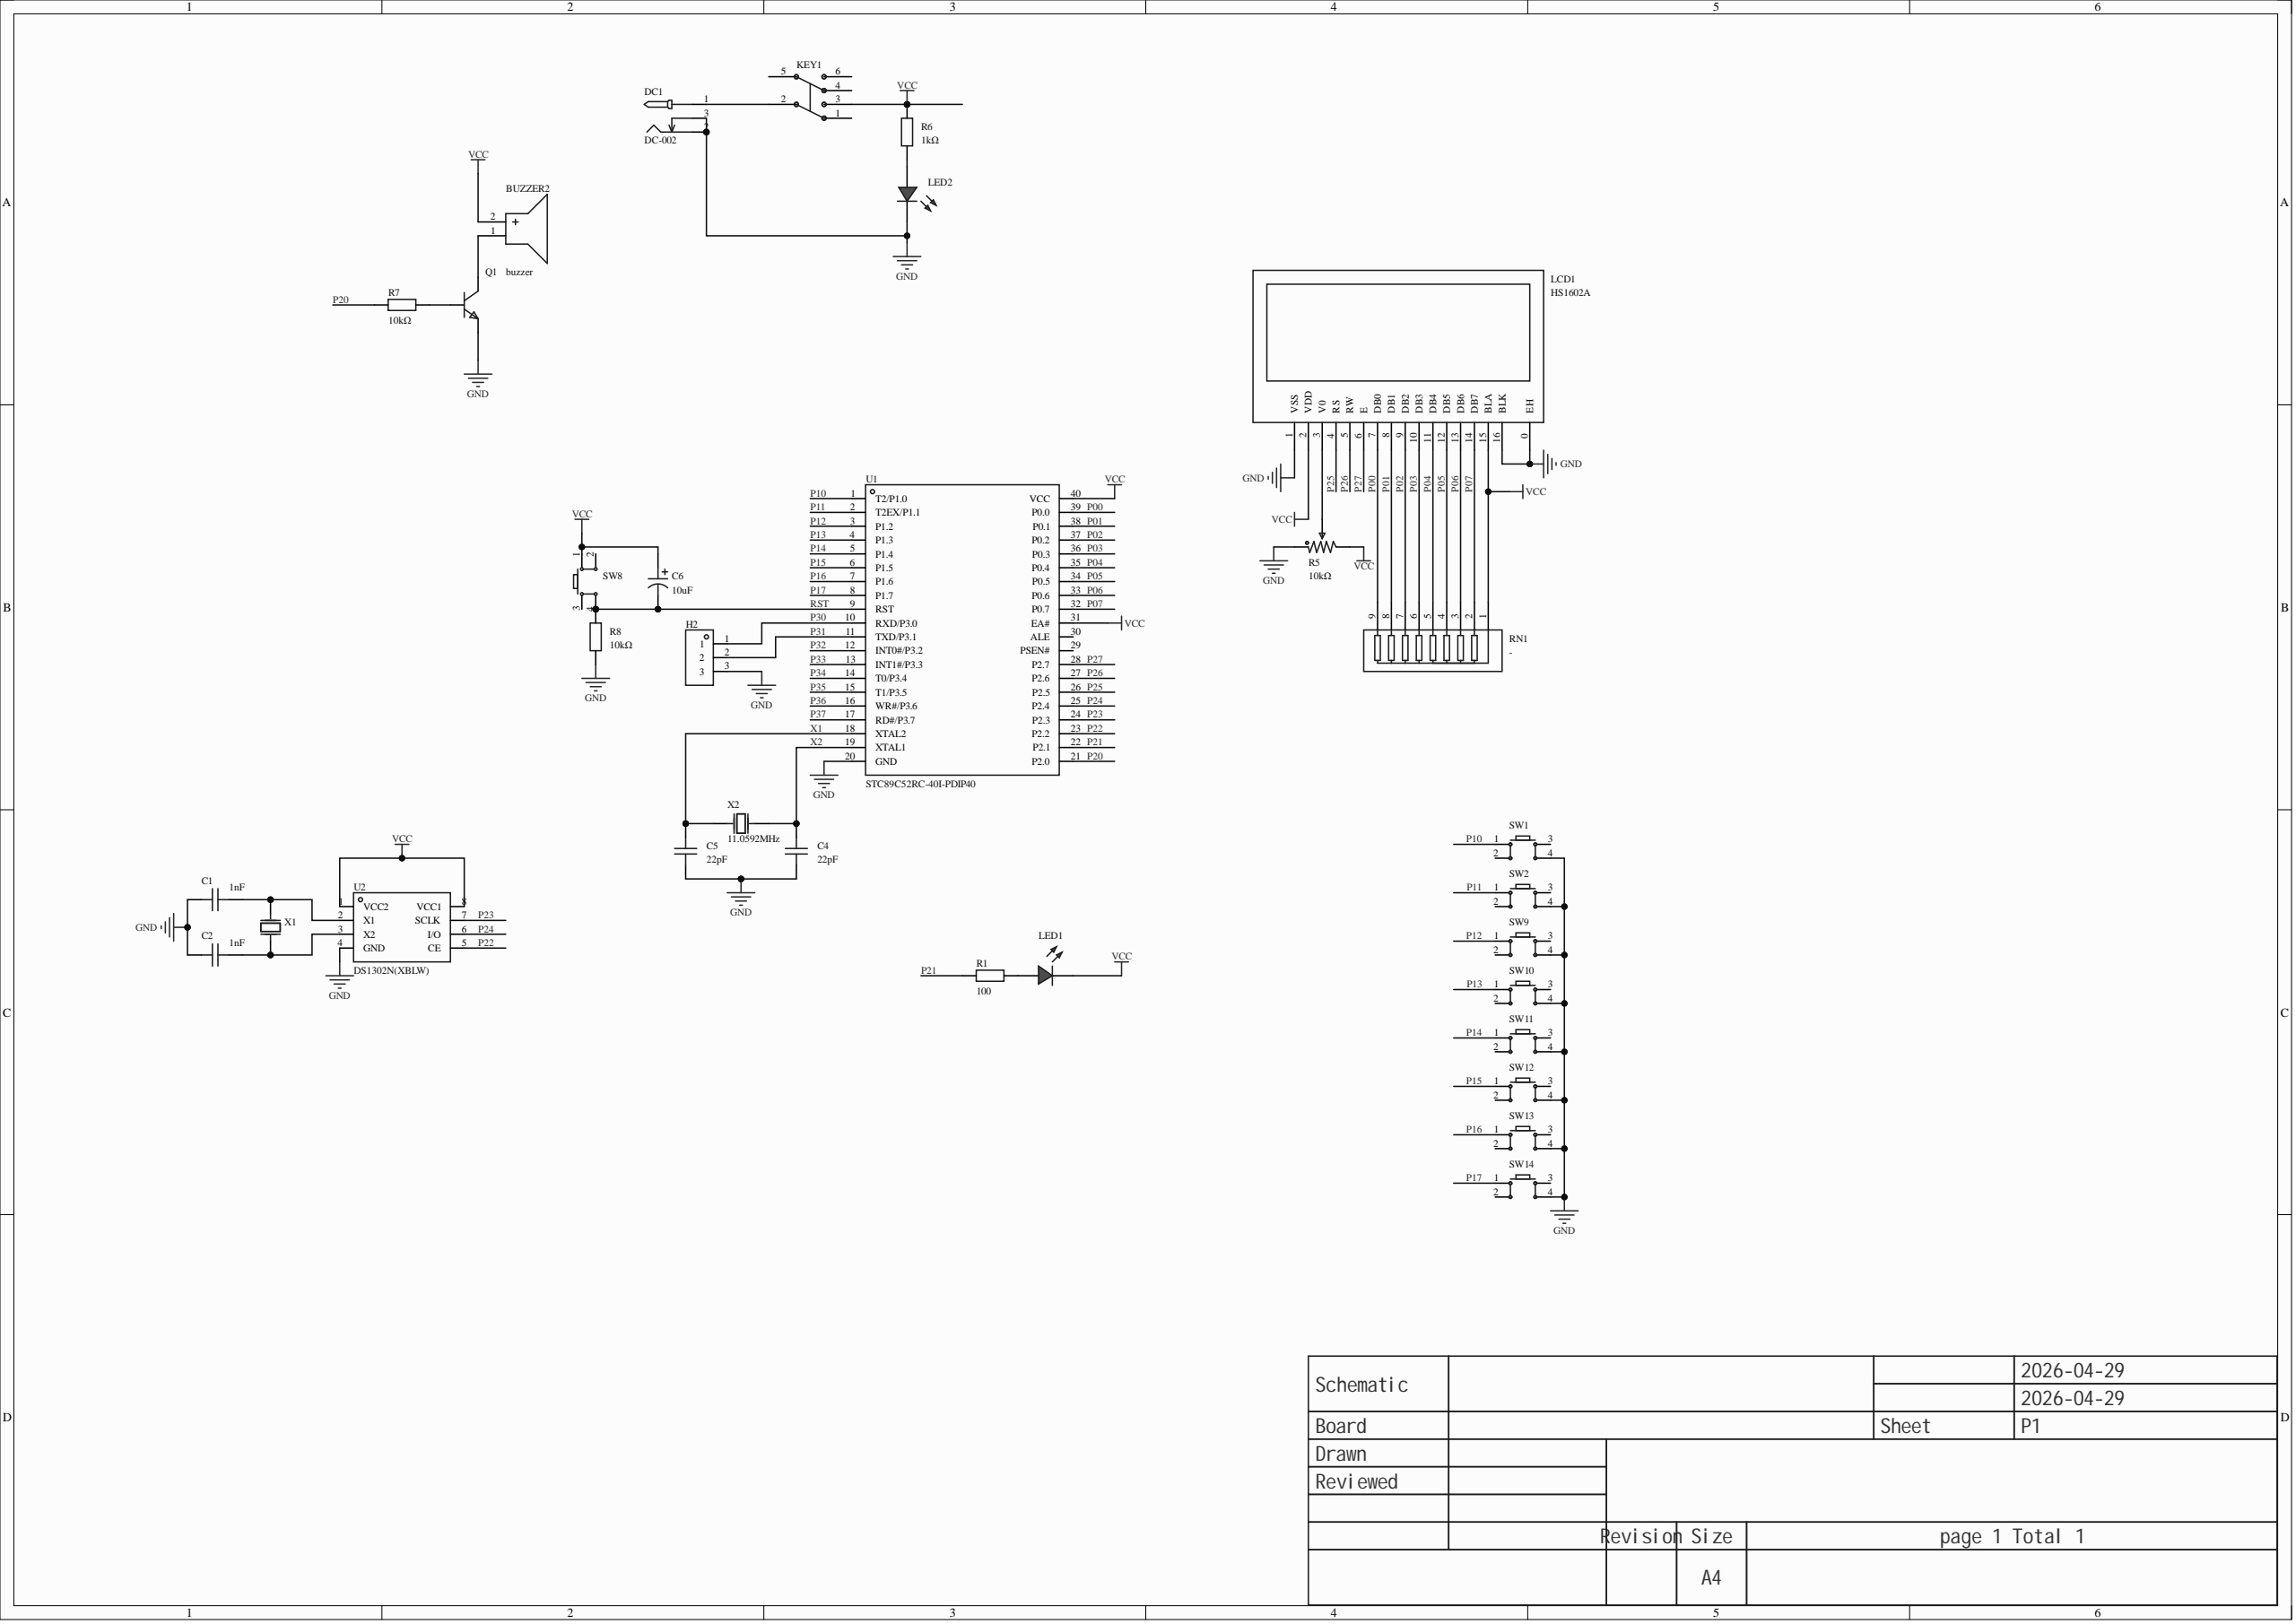Circuit board | Altium Designer | 32 parts | 39 nets
Bill of materials:
Comment,Description,Designator,Footprint,LibRef,Quantity
"buzzer","","BUZZER2","BUZ-TH_BD12.0-P6.00-D0.9-RD","buzzer","1"
"1nF","Capacitance: 30pF; tolerance: ±10%; rated voltage: 25V; temperature coefficient: C0G;","C1, C2","CAP-TH_L3.8-W2.5-P2.54-D0.50","C315C300K3G5TA7301","2"
"22pF","Capacitance: 30pF; tolerance: ±10%; rated voltage: 25V; temperature coefficient: C0G;","C4, C5","CAP-TH_L3.8-W2.5-P2.54-D0.50","C315C300K3G5TA7301","2"
"10uF","Capacitance: 10uF; tolerance: ±20%; rated voltage: 50V; ripple current: 120mA@100KHz; equivalent series resistance (ESR): 1.6Ω;","C6","CAP-TH_BD5.0-P2.00-D0.8-FD-10UF50VC110GL","10UF50VC110GL","1"
"DC-002","","DC1","DC-IN-TH_DC-3510","DC-002","1"
"","","H2","HDR-TH_3P-P2.54-V-M","HDR-M_2.54_1x3P","1"
"Non-latching switch 8.5×8.5 silent","6 pins, 8.5×8.5","KEY1","SW-TH_6P-L8.5-W8.5-P2.54","无自锁开关 8.5×8.5 无声","1"
"HS1602A","Controller chip: SPLC780; size (inch): 2;","LCD1","LCD1602","HS1602A","1"
"","","LED1, LED2","LED_TH-3mm","LED_TH-R_3mm","2"
"","","Q1","S8050_TO_92","S8050_TO_NPN","1"
"100","","R1","Res_1/8W","Res_AXIAL-1/8W","1"
"10kΩ","Resistance: 10kΩ; tolerance: ±25%; power: 100mW;","R5","RES-ADJ-SMD_RM065-V1","RM065-103(10K)","1"
"1kΩ","","R6","Res_1/8W","Res_AXIAL-1/8W","1"
"10kΩ","","R7, R8","Res_1/8W","Res_AXIAL-1/8W","2"
"-","Number of resistors: -; resistance: -; power per element: -;","RN1","RES-ARRAY-TH_9P-P2.54-D1.0","排阻 10 K 5%","1"
"","","SW1, SW2, SW8, SW9, SW10, SW11, SW12, SW13, SW14","SW-TH_4P-L6.0-W6.0-P4.50-LS6.5","Key_TH_6x6x6","9"
"STC89C52RC-40I-PDIP40","CPU core: 51 family; max CPU frequency: -;","U1","DIP-40_L52.0-W13.7-P2.54-LS15.2-BL","STC89C52RC-40I-PDIP40","1"
"DS1302N(XBLW)","Interface type: Three-wire serial interface; crystal: external; alarm output: -;","U2","PDIP-8_L9.3-W6.4-P2.54-LS7.6-BL","DS1302N(XBLW)","1"
"11.059MHz","Crystal type: through-hole crystal; frequency: 11.059MHz; frequency tolerance at room temperature: ±20ppm; load capacitance: 30pF;","X1, X2","OSC-TH_L11.1-W4.7-P4.88","9AC11059302060C3","2"
Netlist (Protel format):
[
BUZZER2
BUZ-TH_BD12.0-P6.00-D0.9-RD
buzzer



]
[
C1
CAP-TH_L3.8-W2.5-P2.54-D0.50
1nF



]
[
C2
CAP-TH_L3.8-W2.5-P2.54-D0.50
1nF



]
[
C4
CAP-TH_L3.8-W2.5-P2.54-D0.50
22pF



]
[
C5
CAP-TH_L3.8-W2.5-P2.54-D0.50
22pF



]
[
C6
CAP-TH_BD5.0-P2.00-D0.8-FD-10UF50VC110GL
10uF



]
[
DC1
DC-IN-TH_DC-3510
DC-002



]
[
H2
HDR-TH_3P-P2.54-V-M




]
[
KEY1
SW-TH_6P-L8.5-W8.5-P2.54
Non-latching switch 8.5×8.5 silent



]
[
LCD1
LCD1602
HS1602A



]
[
LED1
LED_TH-3mm




]
[
LED2
LED_TH-3mm




]
[
Q1
S8050_TO_92




]
[
R1
Res_1/8W
100



]
[
R5
RES-ADJ-SMD_RM065-V1
10kΩ



]
[
R6
Res_1/8W
1kΩ



]
[
R7
Res_1/8W
10kΩ



]
[
R8
Res_1/8W
10kΩ



]
[
RN1
RES-ARRAY-TH_9P-P2.54-D1.0
-



]
[
SW1
SW-TH_4P-L6.0-W6.0-P4.50-LS6.5




]
[
SW2
SW-TH_4P-L6.0-W6.0-P4.50-LS6.5




]
[
SW8
SW-TH_4P-L6.0-W6.0-P4.50-LS6.5




]
[
SW9
SW-TH_4P-L6.0-W6.0-P4.50-LS6.5




]
[
SW10
SW-TH_4P-L6.0-W6.0-P4.50-LS6.5




]
[
SW11
SW-TH_4P-L6.0-W6.0-P4.50-LS6.5




]
[
SW12
SW-TH_4P-L6.0-W6.0-P4.50-LS6.5




]
[
SW13
SW-TH_4P-L6.0-W6.0-P4.50-LS6.5




]
[
SW14
SW-TH_4P-L6.0-W6.0-P4.50-LS6.5




]
[
U1
DIP-40_L52.0-W13.7-P2.54-LS15.2-BL
STC89C52RC-40I-PDIP40



]
[
U2
PDIP-8_L9.3-W6.4-P2.54-LS7.6-BL
DS1302N(XBLW)



]
[
X1
OSC-TH_L11.1-W4.7-P4.88
11.0592MHz



]
[
X2
OSC-TH_L11.1-W4.7-P4.88
11.0592MHz



]
(
X2
C4-2
U1-19
X2-2
)
(
X1
C5-2
U1-18
X2-1
)
(
VCC
BUZZER2-2
C6-1
KEY1-3
LCD1-2
LCD1-15
LED1-2
R5-3
R6-2
RN1-1
SW8-1
U1-31
U1-40
U2-1
U2-8
)
(
RST
C6-2
R8-2
SW8-4
U1-9
)
(
P31
H2-2
U1-11
)
(
P30
H2-1
U1-10
)
(
P27
LCD1-6
U1-28
)
(
P26
LCD1-5
U1-27
)
(
P25
LCD1-4
U1-26
)
(
P24
U1-25
U2-6
)
(
P23
U1-24
U2-7
)
(
P22
U1-23
U2-5
)
(
P21
R1-1
U1-22
)
(
P20
R7-2
U1-21
)
(
P17
SW14-1
U1-8
)
(
P16
SW13-1
U1-7
)
(
P15
SW12-1
U1-6
)
(
P14
SW11-1
U1-5
)
(
P13
SW10-1
U1-4
)
(
P12
SW9-1
U1-3
)
(
P11
SW2-1
U1-2
)
(
P10
SW1-1
U1-1
)
(
P07
LCD1-14
RN1-2
U1-32
)
(
P06
LCD1-13
RN1-3
U1-33
)
(
P05
LCD1-12
RN1-4
U1-34
)
(
P04
LCD1-11
RN1-5
U1-35
)
(
P03
LCD1-10
RN1-6
U1-36
)
(
P02
LCD1-9
RN1-7
U1-37
)
(
P01
LCD1-8
RN1-8
U1-38
)
(
P00
LCD1-7
RN1-9
U1-39
)
(
NetQ1_2
Q1-2
R7-1
)
(
NetLED2_1
LED2-1
R6-1
)
(
NetLED1_1
LED1-1
R1-2
)
(
NetLCD1_3
LCD1-3
R5-2
)
(
NetDC1_1
DC1-1
KEY1-2
)
(
NetC2_1
C2-1
U2-3
X1-1
)
(
NetC1_1
C1-1
U2-2
X1-2
)
(
NetBUZZER2_1
BUZZER2-1
Q1-3
)
(
GND
C1-2
C2-2
C4-1
C5-1
DC1-2
DC1-3
H2-3
LCD1-0
LCD1-1
LCD1-16
LED2-2
Q1-1
R5-1
R8-1
SW1-4
SW2-4
SW9-4
SW10-4
SW11-4
SW12-4
SW13-4
SW14-4
U1-20
U2-4
)